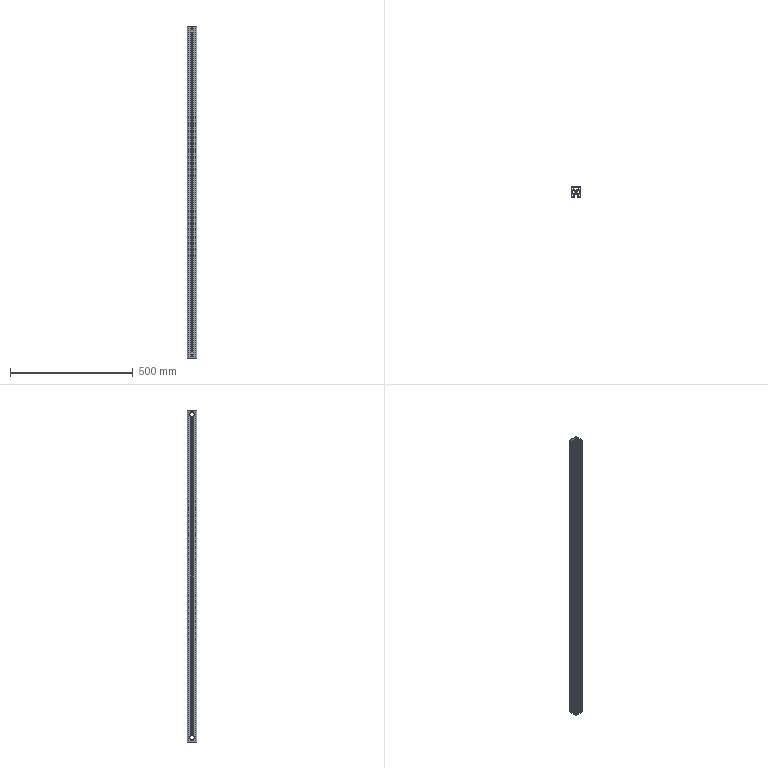Part | SolidWorks | features BaseBody 1, HoleWzd 1, MoveFace 1 | 1 solid | 242 faces | box 40 x 40 x 1350 mm | volume 790915 mm3 | plane 187 | cylinder 55 | commonest cylinder face diameters 6.8 x15 2 x14 19 x12 1 x6 5 x4 9 x4